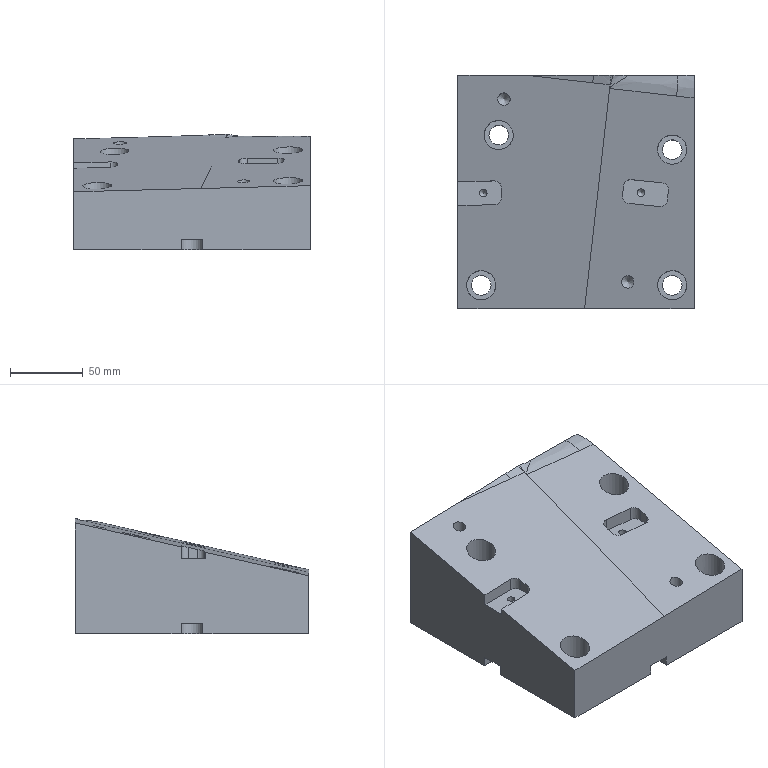Part | NX | features 23 2 | 1 solid | 63 faces | box 162 x 160 x 80.211 mm | volume 1479550 mm3 | plane 29 | cylinder 23 | spline 6 | cone 4 | torus 1 | commonest cylinder face diameters 10 x6 13.5 x4 20 x4 15 x3 5.2 x2 8.5 x2